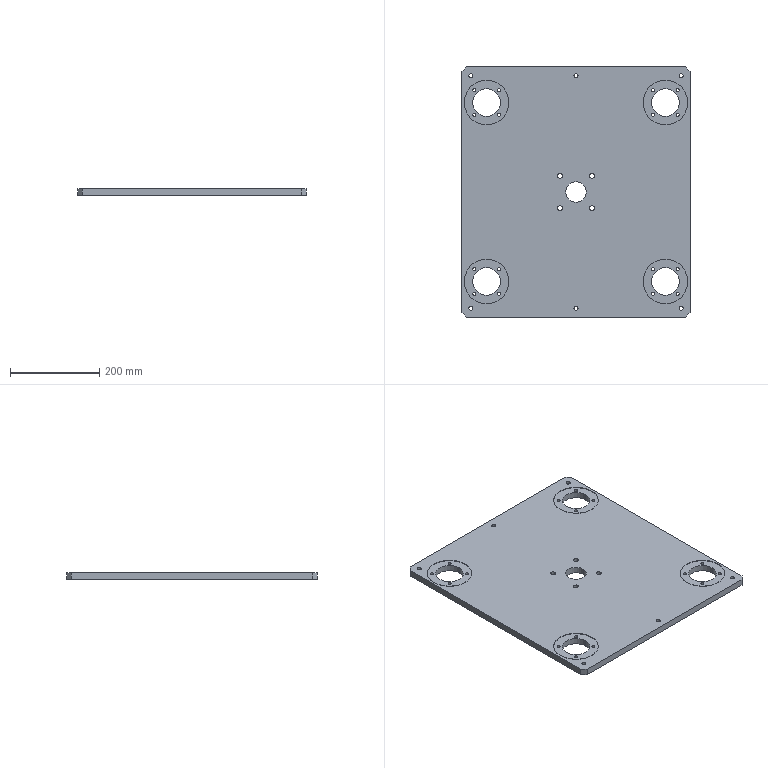Part | SolidWorks | features BaseBody 1 | 1 solid | 84 faces | box 510 x 560 x 15 mm | volume 4036025 mm3 | cylinder 70 | plane 14 | commonest cylinder face diameters 6.8 x32 9 x12 11 x8 62 x8 100 x8 46 x2